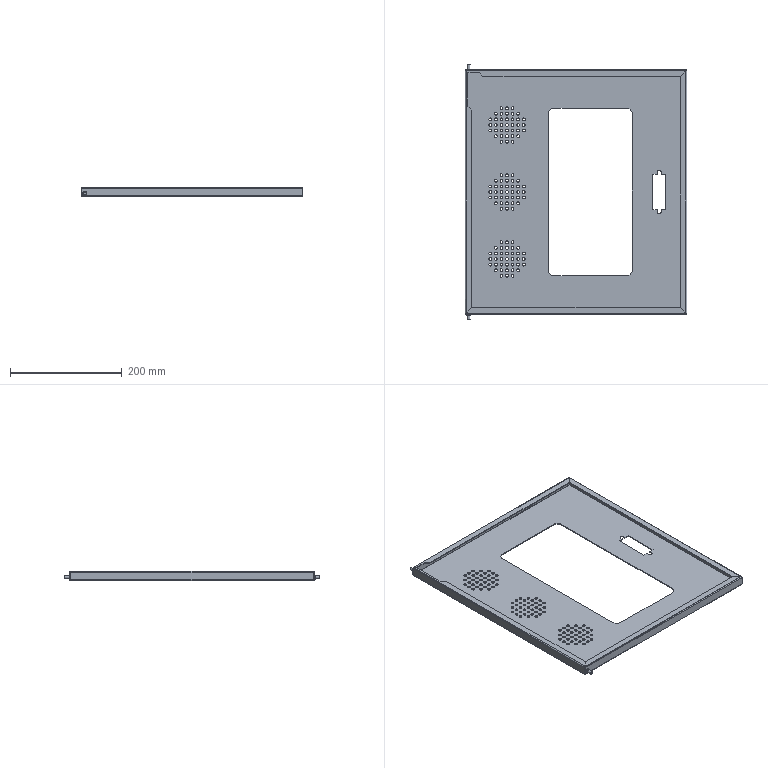Part | STEP file | FHD-021-013-A front door A | 1 solid | 223 faces | box 397 x 457.5 x 17.5 mm | volume 250425 mm3 | cylinder 136 | plane 75 | spline 12 | commonest cylinder face diameters 5 x113 0.4 x8 3.4 x8 20 x4 7 x2 8 x1